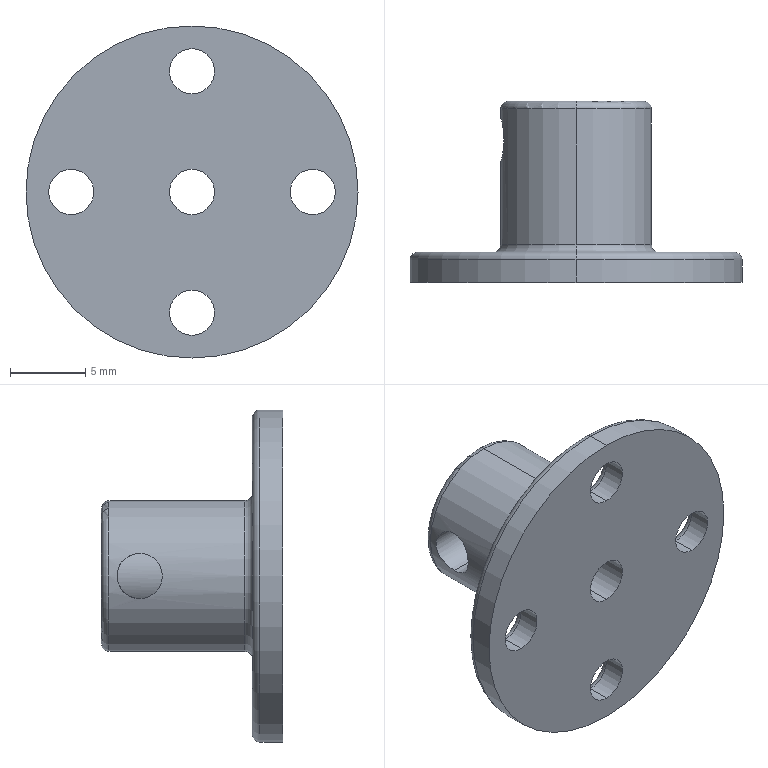Part | STEP file | Flange coupling 3 | 1 solid | 34 faces | box 22 x 12 x 22 mm | volume 1380 mm3 | cylinder 17 | torus 14 | plane 3 | commonest cylinder face diameters 3 x12 10 x2 22 x2 5 x1